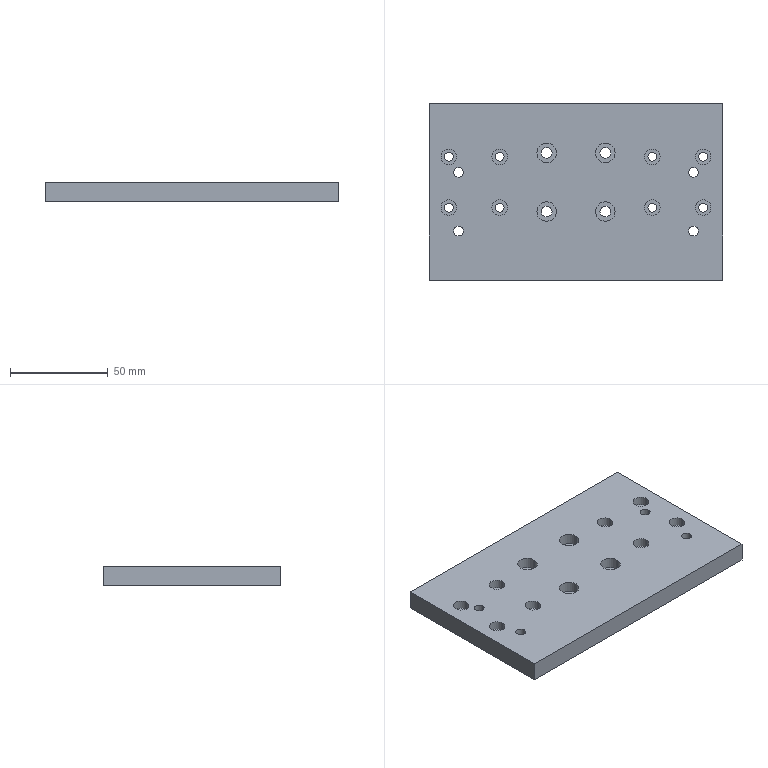Part | STEP file | PN_0036 moving plate | 1 solid | 82 faces | box 150 x 90 x 10 mm | volume 129300 mm3 | cylinder 60 | plane 18 | cone 4 | commonest cylinder face diameters 4.5 x16 8 x16 5 x8 5.5 x8 10 x8 3.3 x4